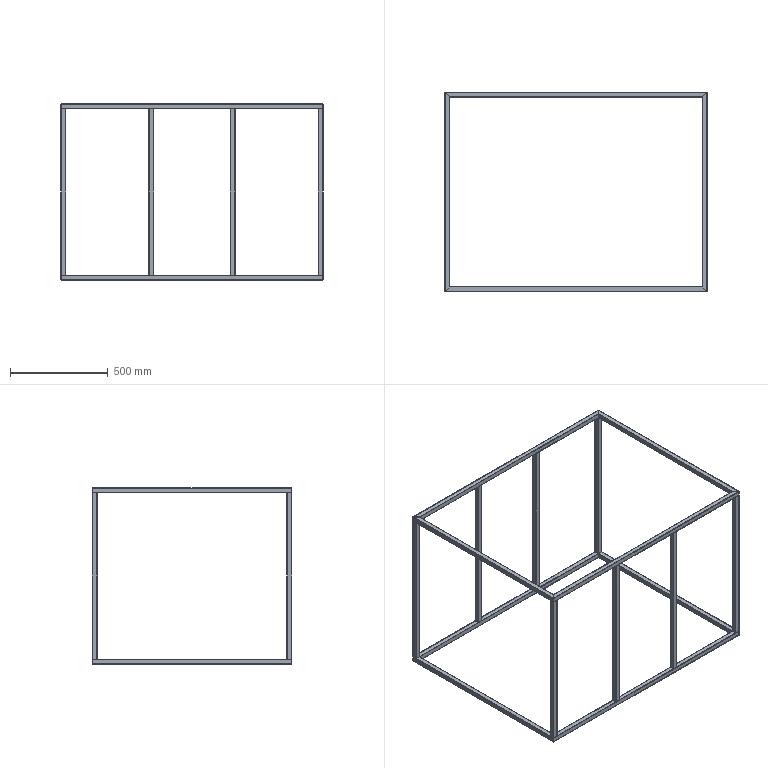Part | SolidWorks | features 3DProfileFeature 1, WeldMemberFeat 1, WeldmentFeature 1 | 16 solids | 288 faces | box 1341 x 1020 x 900 mm | volume 1809729 mm3 | plane 160 | cylinder 128 | commonest cylinder face diameters 0.2 x64 2.6 x64